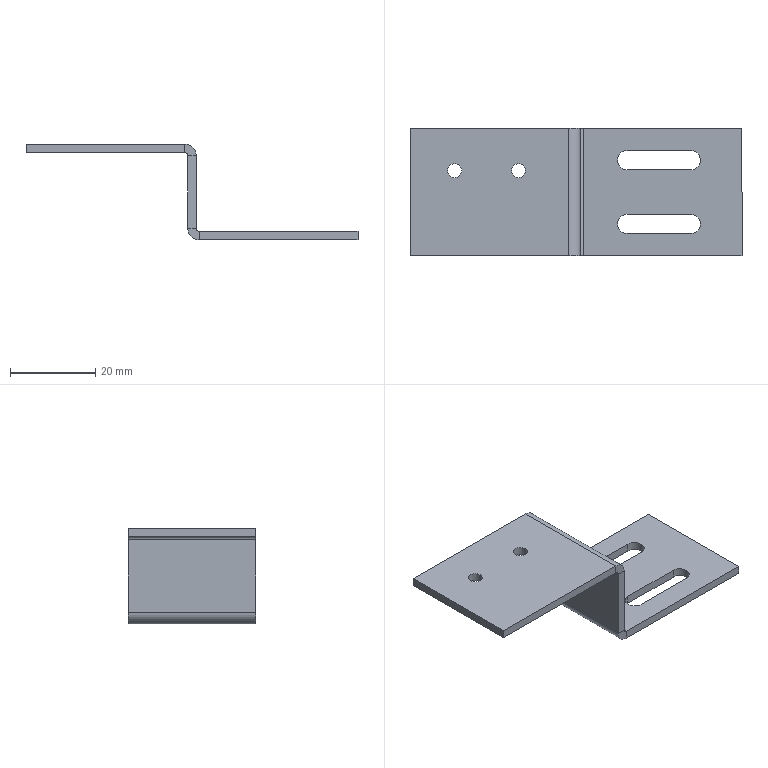Part | SolidWorks | features EdgeFlange 2, FlatPattern 1, HoleWzd 1, ICE 1, SMBaseFlange 1, SheetMetal 1 | 1 solid | 36 faces | box 78 x 30 x 22.5 mm | volume 5453 mm3 | plane 22 | cylinder 14 | commonest cylinder face diameters 4.5 x6 3.3 x4 1.473 x2 5.473 x2
STEP:
#1=CARTESIAN_POINT('',(10.25,-7.5,-2.));
#2=VERTEX_POINT('',#1);
#3=CARTESIAN_POINT('',(8.,-5.25,-2.));
#4=VERTEX_POINT('',#3);
#5=CARTESIAN_POINT('',(8.,-7.5,-2.));
#6=DIRECTION('',(0.,0.,1.));
#7=DIRECTION('',(1.,0.,0.));
#8=AXIS2_PLACEMENT_3D('',#5,#6,#7);
#9=CIRCLE('',#8,2.25);
#10=EDGE_CURVE('',#2,#4,#9,.T.);
#11=ORIENTED_EDGE('',*,*,#10,.F.);
#12=CARTESIAN_POINT('',(10.25,-7.5,0.));
#13=VERTEX_POINT('',#12);
#14=CARTESIAN_POINT('',(10.25,-7.5,-2.));
#15=DIRECTION('',(0.,0.,1.));
#16=VECTOR('',#15,1000.);
#17=LINE('',#14,#16);
#18=EDGE_CURVE('',#2,#13,#17,.T.);
#19=ORIENTED_EDGE('',*,*,#18,.T.);
#20=CARTESIAN_POINT('',(8.,-5.25,0.));
#21=VERTEX_POINT('',#20);
#22=CARTESIAN_POINT('',(8.,-7.5,0.));
#23=DIRECTION('',(0.,0.,1.));
#24=DIRECTION('',(1.,0.,0.));
#25=AXIS2_PLACEMENT_3D('',#22,#23,#24);
#26=CIRCLE('',#25,2.25);
#27=EDGE_CURVE('',#13,#21,#26,.T.);
#28=ORIENTED_EDGE('',*,*,#27,.T.);
#29=CARTESIAN_POINT('',(8.,-5.25,-2.));
#30=DIRECTION('',(0.,0.,1.));
#31=VECTOR('',#30,1000.);
#32=LINE('',#29,#31);
#33=EDGE_CURVE('',#4,#21,#32,.T.);
#34=ORIENTED_EDGE('',*,*,#33,.F.);
#35=EDGE_LOOP('',(#11,#19,#28,#34));
#36=FACE_OUTER_BOUND('',#35,.T.);
#37=CARTESIAN_POINT('',(8.,-7.5,-2.));
#38=DIRECTION('',(0.,0.,1.));
#39=DIRECTION('',(1.,0.,0.));
#40=AXIS2_PLACEMENT_3D('',#37,#38,#39);
#41=CYLINDRICAL_SURFACE('',#40,2.25);
#42=ADVANCED_FACE('',(#36),#41,.F.);
#43=CARTESIAN_POINT('',(10.25,7.5,-2.));
#44=VERTEX_POINT('',#43);
#45=CARTESIAN_POINT('',(8.,9.75,-2.));
#46=VERTEX_POINT('',#45);
#47=CARTESIAN_POINT('',(8.,7.5,-2.));
#48=DIRECTION('',(0.,0.,1.));
#49=DIRECTION('',(1.,0.,0.));
#50=AXIS2_PLACEMENT_3D('',#47,#48,#49);
#51=CIRCLE('',#50,2.25);
#52=EDGE_CURVE('',#44,#46,#51,.T.);
#53=ORIENTED_EDGE('',*,*,#52,.F.);
#54=CARTESIAN_POINT('',(10.25,7.5,0.));
#55=VERTEX_POINT('',#54);
#56=CARTESIAN_POINT('',(10.25,7.5,-2.));
#57=DIRECTION('',(0.,0.,1.));
#58=VECTOR('',#57,1000.);
#59=LINE('',#56,#58);
#60=EDGE_CURVE('',#44,#55,#59,.T.);
#61=ORIENTED_EDGE('',*,*,#60,.T.);
#62=CARTESIAN_POINT('',(8.,9.75,0.));
#63=VERTEX_POINT('',#62);
#64=CARTESIAN_POINT('',(8.,7.5,0.));
#65=DIRECTION('',(0.,0.,1.));
#66=DIRECTION('',(1.,0.,0.));
#67=AXIS2_PLACEMENT_3D('',#64,#65,#66);
#68=CIRCLE('',#67,2.25);
#69=EDGE_CURVE('',#55,#63,#68,.T.);
#70=ORIENTED_EDGE('',*,*,#69,.T.);
#71=CARTESIAN_POINT('',(8.,9.75,-2.));
#72=DIRECTION('',(0.,0.,1.));
#73=VECTOR('',#72,1000.);
#74=LINE('',#71,#73);
#75=EDGE_CURVE('',#46,#63,#74,.T.);
#76=ORIENTED_EDGE('',*,*,#75,.F.);
#77=EDGE_LOOP('',(#53,#61,#70,#76));
#78=FACE_OUTER_BOUND('',#77,.T.);
#79=CARTESIAN_POINT('',(8.,7.5,-2.));
#80=DIRECTION('',(0.,0.,1.));
#81=DIRECTION('',(1.,0.,0.));
#82=AXIS2_PLACEMENT_3D('',#79,#80,#81);
#83=CYLINDRICAL_SURFACE('',#82,2.25);
#84=ADVANCED_FACE('',(#78),#83,.F.);
#85=CARTESIAN_POINT('',(-45.85,5.,18.5));
#86=VERTEX_POINT('',#85);
#87=CARTESIAN_POINT('',(-49.15,5.,18.5));
#88=VERTEX_POINT('',#87);
#89=CARTESIAN_POINT('',(-47.5,5.,18.5));
#90=DIRECTION('',(0.,0.,-1.));
#91=DIRECTION('',(-1.,0.,0.));
#92=AXIS2_PLACEMENT_3D('',#89,#90,#91);
#93=CIRCLE('',#92,1.65);
#94=EDGE_CURVE('',#86,#88,#93,.T.);
#95=ORIENTED_EDGE('',*,*,#94,.T.);
#96=CARTESIAN_POINT('',(-49.15,5.,20.5));
#97=VERTEX_POINT('',#96);
#98=CARTESIAN_POINT('',(-49.15,5.,20.5));
#99=DIRECTION('',(0.,0.,1.));
#100=VECTOR('',#99,1000.);
#101=LINE('',#98,#100);
#102=EDGE_CURVE('',#88,#97,#101,.T.);
#103=ORIENTED_EDGE('',*,*,#102,.T.);
#104=CARTESIAN_POINT('',(-45.85,5.,20.5));
#105=VERTEX_POINT('',#104);
#106=CARTESIAN_POINT('',(-47.5,5.,20.5));
#107=DIRECTION('',(0.,0.,1.));
#108=DIRECTION('',(1.,0.,0.));
#109=AXIS2_PLACEMENT_3D('',#106,#107,#108);
#110=CIRCLE('',#109,1.65);
#111=EDGE_CURVE('',#97,#105,#110,.T.);
#112=ORIENTED_EDGE('',*,*,#111,.T.);
#113=CARTESIAN_POINT('',(-45.85,5.,20.5));
#114=DIRECTION('',(0.,0.,1.));
#115=VECTOR('',#114,1000.);
#116=LINE('',#113,#115);
#117=EDGE_CURVE('',#86,#105,#116,.T.);
#118=ORIENTED_EDGE('',*,*,#117,.F.);
#119=EDGE_LOOP('',(#95,#103,#112,#118));
#120=FACE_OUTER_BOUND('',#119,.T.);
#121=CARTESIAN_POINT('',(-47.5,5.,20.5));
#122=DIRECTION('',(0.,0.,1.));
#123=DIRECTION('',(1.,0.,0.));
#124=AXIS2_PLACEMENT_3D('',#121,#122,#123);
#125=CYLINDRICAL_SURFACE('',#124,1.65);
#126=ADVANCED_FACE('',(#120),#125,.F.);
#127=CARTESIAN_POINT('',(-30.85,5.,18.5));
#128=VERTEX_POINT('',#127);
#129=CARTESIAN_POINT('',(-34.15,5.,18.5));
#130=VERTEX_POINT('',#129);
#131=CARTESIAN_POINT('',(-32.5,5.,18.5));
#132=DIRECTION('',(0.,0.,-1.));
#133=DIRECTION('',(-1.,0.,0.));
#134=AXIS2_PLACEMENT_3D('',#131,#132,#133);
#135=CIRCLE('',#134,1.65);
#136=EDGE_CURVE('',#128,#130,#135,.T.);
#137=ORIENTED_EDGE('',*,*,#136,.T.);
#138=CARTESIAN_POINT('',(-34.15,5.,20.5));
#139=VERTEX_POINT('',#138);
#140=CARTESIAN_POINT('',(-34.15,5.,20.5));
#141=DIRECTION('',(0.,0.,1.));
#142=VECTOR('',#141,1000.);
#143=LINE('',#140,#142);
#144=EDGE_CURVE('',#130,#139,#143,.T.);
#145=ORIENTED_EDGE('',*,*,#144,.T.);
#146=CARTESIAN_POINT('',(-30.85,5.,20.5));
#147=VERTEX_POINT('',#146);
#148=CARTESIAN_POINT('',(-32.5,5.,20.5));
#149=DIRECTION('',(0.,0.,1.));
#150=DIRECTION('',(1.,0.,0.));
#151=AXIS2_PLACEMENT_3D('',#148,#149,#150);
#152=CIRCLE('',#151,1.65);
#153=EDGE_CURVE('',#139,#147,#152,.T.);
#154=ORIENTED_EDGE('',*,*,#153,.T.);
#155=CARTESIAN_POINT('',(-30.85,5.,20.5));
#156=DIRECTION('',(0.,0.,1.));
#157=VECTOR('',#156,1000.);
#158=LINE('',#155,#157);
#159=EDGE_CURVE('',#128,#147,#158,.T.);
#160=ORIENTED_EDGE('',*,*,#159,.F.);
#161=EDGE_LOOP('',(#137,#145,#154,#160));
#162=FACE_OUTER_BOUND('',#161,.T.);
#163=CARTESIAN_POINT('',(-32.5,5.,20.5));
#164=DIRECTION('',(0.,0.,1.));
#165=DIRECTION('',(1.,0.,0.));
#166=AXIS2_PLACEMENT_3D('',#163,#164,#165);
#167=CYLINDRICAL_SURFACE('',#166,1.65);
#168=ADVANCED_FACE('',(#162),#167,.F.);
#169=CARTESIAN_POINT('',(-20.,15.,0.7366));
#170=VERTEX_POINT('',#169);
#171=CARTESIAN_POINT('',(-20.,15.,17.763));
#172=VERTEX_POINT('',#171);
#173=CARTESIAN_POINT('',(-20.,15.,20.5));
#174=DIRECTION('',(0.,0.,1.));
#175=VECTOR('',#174,1000.);
#176=LINE('',#173,#175);
#177=EDGE_CURVE('',#170,#172,#176,.T.);
#178=ORIENTED_EDGE('',*,*,#177,.T.);
#179=CARTESIAN_POINT('',(-18.,15.,17.763));
#180=VERTEX_POINT('',#179);
#181=CARTESIAN_POINT('',(-20.,15.,17.763));
#182=DIRECTION('',(1.,0.,0.));
#183=VECTOR('',#182,1000.);
#184=LINE('',#181,#183);
#185=EDGE_CURVE('',#172,#180,#184,.T.);
#186=ORIENTED_EDGE('',*,*,#185,.T.);
#187=CARTESIAN_POINT('',(-18.,15.,0.7366));
#188=VERTEX_POINT('',#187);
#189=CARTESIAN_POINT('',(-18.,15.,0.));
#190=DIRECTION('',(0.,0.,1.));
#191=VECTOR('',#190,1000.);
#192=LINE('',#189,#191);
#193=EDGE_CURVE('',#188,#180,#192,.T.);
#194=ORIENTED_EDGE('',*,*,#193,.F.);
#195=CARTESIAN_POINT('',(-20.,15.,0.7366));
#196=DIRECTION('',(-1.,0.,0.));
#197=VECTOR('',#196,1000.);
#198=LINE('',#195,#197);
#199=EDGE_CURVE('',#188,#170,#198,.T.);
#200=ORIENTED_EDGE('',*,*,#199,.T.);
#201=EDGE_LOOP('',(#178,#186,#194,#200));
#202=FACE_OUTER_BOUND('',#201,.T.);
#203=CARTESIAN_POINT('',(-20.,15.,20.5));
#204=DIRECTION('',(0.,1.,0.));
#205=DIRECTION('',(0.,0.,1.));
#206=AXIS2_PLACEMENT_3D('',#203,#204,#205);
#207=PLANE('',#206);
#208=ADVANCED_FACE('',(#202),#207,.T.);
#209=CARTESIAN_POINT('',(-20.,-15.,17.763));
#210=VERTEX_POINT('',#209);
#211=CARTESIAN_POINT('',(-20.,-15.,0.7366));
#212=VERTEX_POINT('',#211);
#213=CARTESIAN_POINT('',(-20.,-15.,0.));
#214=DIRECTION('',(0.,0.,-1.));
#215=VECTOR('',#214,1000.);
#216=LINE('',#213,#215);
#217=EDGE_CURVE('',#210,#212,#216,.T.);
#218=ORIENTED_EDGE('',*,*,#217,.F.);
#219=CARTESIAN_POINT('',(-20.,15.,17.763));
#220=DIRECTION('',(0.,-1.,0.));
#221=VECTOR('',#220,1000.);
#222=LINE('',#219,#221);
#223=EDGE_CURVE('',#172,#210,#222,.T.);
#224=ORIENTED_EDGE('',*,*,#223,.F.);
#225=ORIENTED_EDGE('',*,*,#177,.F.);
#226=CARTESIAN_POINT('',(-20.,0.,0.7366));
#227=DIRECTION('',(0.,-1.,0.));
#228=VECTOR('',#227,1000.);
#229=LINE('',#226,#228);
#230=EDGE_CURVE('',#170,#212,#229,.T.);
#231=ORIENTED_EDGE('',*,*,#230,.T.);
#232=EDGE_LOOP('',(#218,#224,#225,#231));
#233=FACE_OUTER_BOUND('',#232,.T.);
#234=CARTESIAN_POINT('',(-20.,0.,0.));
#235=DIRECTION('',(-1.,0.,0.));
#236=DIRECTION('',(0.,0.,1.));
#237=AXIS2_PLACEMENT_3D('',#234,#235,#236);
#238=PLANE('',#237);
#239=ADVANCED_FACE('',(#233),#238,.T.);
#240=CARTESIAN_POINT('',(-18.,-15.,17.763));
#241=VERTEX_POINT('',#240);
#242=CARTESIAN_POINT('',(-18.,15.,17.763));
#243=DIRECTION('',(0.,-1.,0.));
#244=VECTOR('',#243,1000.);
#245=LINE('',#242,#244);
#246=EDGE_CURVE('',#180,#241,#245,.T.);
#247=ORIENTED_EDGE('',*,*,#246,.T.);
#248=CARTESIAN_POINT('',(-18.,-15.,0.7366));
#249=VERTEX_POINT('',#248);
#250=CARTESIAN_POINT('',(-18.,-15.,0.));
#251=DIRECTION('',(0.,0.,-1.));
#252=VECTOR('',#251,1000.);
#253=LINE('',#250,#252);
#254=EDGE_CURVE('',#241,#249,#253,.T.);
#255=ORIENTED_EDGE('',*,*,#254,.T.);
#256=CARTESIAN_POINT('',(-18.,15.,0.7366));
#257=DIRECTION('',(0.,-1.,0.));
#258=VECTOR('',#257,1000.);
#259=LINE('',#256,#258);
#260=EDGE_CURVE('',#188,#249,#259,.T.);
#261=ORIENTED_EDGE('',*,*,#260,.F.);
#262=ORIENTED_EDGE('',*,*,#193,.T.);
#263=EDGE_LOOP('',(#247,#255,#261,#262));
#264=FACE_OUTER_BOUND('',#263,.T.);
#265=CARTESIAN_POINT('',(-18.,0.,0.));
#266=DIRECTION('',(-1.,0.,0.));
#267=DIRECTION('',(0.,0.,1.));
#268=AXIS2_PLACEMENT_3D('',#265,#266,#267);
#269=PLANE('',#268);
#270=ADVANCED_FACE('',(#264),#269,.F.);
#271=CARTESIAN_POINT('',(-17.263,-15.,0.));
#272=VERTEX_POINT('',#271);
#273=CARTESIAN_POINT('',(20.,-15.,0.));
#274=VERTEX_POINT('',#273);
#275=CARTESIAN_POINT('',(-20.,-15.,0.));
#276=DIRECTION('',(1.,0.,0.));
#277=VECTOR('',#276,1000.);
#278=LINE('',#275,#277);
#279=EDGE_CURVE('',#272,#274,#278,.T.);
#280=ORIENTED_EDGE('',*,*,#279,.F.);
#281=CARTESIAN_POINT('',(-17.263,-15.,-2.));
#282=VERTEX_POINT('',#281);
#283=CARTESIAN_POINT('',(-17.263,-15.,0.));
#284=DIRECTION('',(0.,0.,-1.));
#285=VECTOR('',#284,1000.);
#286=LINE('',#283,#285);
#287=EDGE_CURVE('',#272,#282,#286,.T.);
#288=ORIENTED_EDGE('',*,*,#287,.T.);
#289=CARTESIAN_POINT('',(20.,-15.,-2.));
#290=VERTEX_POINT('',#289);
#291=CARTESIAN_POINT('',(-20.,-15.,-2.));
#292=DIRECTION('',(1.,0.,0.));
#293=VECTOR('',#292,1000.);
#294=LINE('',#291,#293);
#295=EDGE_CURVE('',#282,#290,#294,.T.);
#296=ORIENTED_EDGE('',*,*,#295,.T.);
#297=CARTESIAN_POINT('',(20.,-15.,-2.));
#298=DIRECTION('',(0.,0.,1.));
#299=VECTOR('',#298,1000.);
#300=LINE('',#297,#299);
#301=EDGE_CURVE('',#290,#274,#300,.T.);
#302=ORIENTED_EDGE('',*,*,#301,.T.);
#303=EDGE_LOOP('',(#280,#288,#296,#302));
#304=FACE_OUTER_BOUND('',#303,.T.);
#305=CARTESIAN_POINT('',(-20.,-15.,-2.));
#306=DIRECTION('',(0.,-1.,0.));
#307=DIRECTION('',(0.,0.,-1.));
#308=AXIS2_PLACEMENT_3D('',#305,#306,#307);
#309=PLANE('',#308);
#310=ADVANCED_FACE('',(#304),#309,.T.);
#311=CARTESIAN_POINT('',(-7.,-5.25,-2.));
#312=VERTEX_POINT('',#311);
#313=CARTESIAN_POINT('',(-7.,-5.25,-2.));
#314=DIRECTION('',(-1.,0.,0.));
#315=VECTOR('',#314,1000.);
#316=LINE('',#313,#315);
#317=EDGE_CURVE('',#4,#312,#316,.T.);
#318=ORIENTED_EDGE('',*,*,#317,.T.);
#319=CARTESIAN_POINT('',(-7.,-9.75,-2.));
#320=VERTEX_POINT('',#319);
#321=CARTESIAN_POINT('',(-7.,-7.5,-2.));
#322=DIRECTION('',(0.,0.,1.));
#323=DIRECTION('',(1.,0.,0.));
#324=AXIS2_PLACEMENT_3D('',#321,#322,#323);
#325=CIRCLE('',#324,2.25);
#326=EDGE_CURVE('',#312,#320,#325,.T.);
#327=ORIENTED_EDGE('',*,*,#326,.T.);
#328=CARTESIAN_POINT('',(8.,-9.75,-2.));
#329=VERTEX_POINT('',#328);
#330=CARTESIAN_POINT('',(-7.,-9.75,-2.));
#331=DIRECTION('',(1.,0.,0.));
#332=VECTOR('',#331,1000.);
#333=LINE('',#330,#332);
#334=EDGE_CURVE('',#320,#329,#333,.T.);
#335=ORIENTED_EDGE('',*,*,#334,.T.);
#336=CARTESIAN_POINT('',(8.,-7.5,-2.));
#337=DIRECTION('',(0.,0.,1.));
#338=DIRECTION('',(1.,0.,0.));
#339=AXIS2_PLACEMENT_3D('',#336,#337,#338);
#340=CIRCLE('',#339,2.25);
#341=EDGE_CURVE('',#329,#2,#340,.T.);
#342=ORIENTED_EDGE('',*,*,#341,.T.);
#343=ORIENTED_EDGE('',*,*,#10,.T.);
#344=EDGE_LOOP('',(#318,#327,#335,#342,#343));
#345=FACE_BOUND('',#344,.T.);
#346=CARTESIAN_POINT('',(-7.,9.75,-2.));
#347=VERTEX_POINT('',#346);
#348=CARTESIAN_POINT('',(-7.,9.75,-2.));
#349=DIRECTION('',(-1.,0.,0.));
#350=VECTOR('',#349,1000.);
#351=LINE('',#348,#350);
#352=EDGE_CURVE('',#46,#347,#351,.T.);
#353=ORIENTED_EDGE('',*,*,#352,.T.);
#354=CARTESIAN_POINT('',(-7.,5.25,-2.));
#355=VERTEX_POINT('',#354);
#356=CARTESIAN_POINT('',(-7.,7.5,-2.));
#357=DIRECTION('',(0.,0.,1.));
#358=DIRECTION('',(1.,0.,0.));
#359=AXIS2_PLACEMENT_3D('',#356,#357,#358);
#360=CIRCLE('',#359,2.25);
#361=EDGE_CURVE('',#347,#355,#360,.T.);
#362=ORIENTED_EDGE('',*,*,#361,.T.);
#363=CARTESIAN_POINT('',(8.,5.25,-2.));
#364=VERTEX_POINT('',#363);
#365=CARTESIAN_POINT('',(-7.,5.25,-2.));
#366=DIRECTION('',(1.,0.,0.));
#367=VECTOR('',#366,1000.);
#368=LINE('',#365,#367);
#369=EDGE_CURVE('',#355,#364,#368,.T.);
#370=ORIENTED_EDGE('',*,*,#369,.T.);
#371=CARTESIAN_POINT('',(8.,7.5,-2.));
#372=DIRECTION('',(0.,0.,1.));
#373=DIRECTION('',(1.,0.,0.));
#374=AXIS2_PLACEMENT_3D('',#371,#372,#373);
#375=CIRCLE('',#374,2.25);
#376=EDGE_CURVE('',#364,#44,#375,.T.);
#377=ORIENTED_EDGE('',*,*,#376,.T.);
#378=ORIENTED_EDGE('',*,*,#52,.T.);
#379=EDGE_LOOP('',(#353,#362,#370,#377,#378));
#380=FACE_BOUND('',#379,.T.);
#381=CARTESIAN_POINT('',(-17.263,15.,-2.));
#382=VERTEX_POINT('',#381);
#383=CARTESIAN_POINT('',(-17.263,-15.,-2.));
#384=DIRECTION('',(0.,1.,0.));
#385=VECTOR('',#384,1000.);
#386=LINE('',#383,#385);
#387=EDGE_CURVE('',#282,#382,#386,.T.);
#388=ORIENTED_EDGE('',*,*,#387,.T.);
#389=CARTESIAN_POINT('',(20.,15.,-2.));
#390=VERTEX_POINT('',#389);
#391=CARTESIAN_POINT('',(-20.,15.,-2.));
#392=DIRECTION('',(-1.,0.,0.));
#393=VECTOR('',#392,1000.);
#394=LINE('',#391,#393);
#395=EDGE_CURVE('',#390,#382,#394,.T.);
#396=ORIENTED_EDGE('',*,*,#395,.F.);
#397=CARTESIAN_POINT('',(20.,15.,-2.));
#398=DIRECTION('',(0.,1.,0.));
#399=VECTOR('',#398,1000.);
#400=LINE('',#397,#399);
#401=EDGE_CURVE('',#290,#390,#400,.T.);
#402=ORIENTED_EDGE('',*,*,#401,.F.);
#403=ORIENTED_EDGE('',*,*,#295,.F.);
#404=EDGE_LOOP('',(#388,#396,#402,#403));
#405=FACE_OUTER_BOUND('',#404,.T.);
#406=CARTESIAN_POINT('',(0.,0.,-2.));
#407=DIRECTION('',(0.,0.,1.));
#408=DIRECTION('',(1.,0.,0.));
#409=AXIS2_PLACEMENT_3D('',#406,#407,#408);
#410=PLANE('',#409);
#411=ADVANCED_FACE('',(#345,#380,#405),#410,.F.);
#412=CARTESIAN_POINT('',(-7.,-5.25,0.));
#413=VERTEX_POINT('',#412);
#414=CARTESIAN_POINT('',(-7.,-9.75,0.));
#415=VERTEX_POINT('',#414);
#416=CARTESIAN_POINT('',(-7.,-7.5,0.));
#417=DIRECTION('',(0.,0.,1.));
#418=DIRECTION('',(1.,0.,0.));
#419=AXIS2_PLACEMENT_3D('',#416,#417,#418);
#420=CIRCLE('',#419,2.25);
#421=EDGE_CURVE('',#413,#415,#420,.T.);
#422=ORIENTED_EDGE('',*,*,#421,.F.);
#423=CARTESIAN_POINT('',(-7.,-5.25,0.));
#424=DIRECTION('',(-1.,0.,0.));
#425=VECTOR('',#424,1000.);
#426=LINE('',#423,#425);
#427=EDGE_CURVE('',#21,#413,#426,.T.);
#428=ORIENTED_EDGE('',*,*,#427,.F.);
#429=ORIENTED_EDGE('',*,*,#27,.F.);
#430=CARTESIAN_POINT('',(8.,-9.75,0.));
#431=VERTEX_POINT('',#430);
#432=CARTESIAN_POINT('',(8.,-7.5,0.));
#433=DIRECTION('',(0.,0.,1.));
#434=DIRECTION('',(1.,0.,0.));
#435=AXIS2_PLACEMENT_3D('',#432,#433,#434);
#436=CIRCLE('',#435,2.25);
#437=EDGE_CURVE('',#431,#13,#436,.T.);
#438=ORIENTED_EDGE('',*,*,#437,.F.);
#439=CARTESIAN_POINT('',(-7.,-9.75,0.));
#440=DIRECTION('',(1.,0.,0.));
#441=VECTOR('',#440,1000.);
#442=LINE('',#439,#441);
#443=EDGE_CURVE('',#415,#431,#442,.T.);
#444=ORIENTED_EDGE('',*,*,#443,.F.);
#445=EDGE_LOOP('',(#422,#428,#429,#438,#444));
#446=FACE_BOUND('',#445,.T.);
#447=CARTESIAN_POINT('',(-7.,9.75,0.));
#448=VERTEX_POINT('',#447);
#449=CARTESIAN_POINT('',(-7.,5.25,0.));
#450=VERTEX_POINT('',#449);
#451=CARTESIAN_POINT('',(-7.,7.5,0.));
#452=DIRECTION('',(0.,0.,1.));
#453=DIRECTION('',(1.,0.,0.));
#454=AXIS2_PLACEMENT_3D('',#451,#452,#453);
#455=CIRCLE('',#454,2.25);
#456=EDGE_CURVE('',#448,#450,#455,.T.);
#457=ORIENTED_EDGE('',*,*,#456,.F.);
#458=CARTESIAN_POINT('',(-7.,9.75,0.));
#459=DIRECTION('',(-1.,0.,0.));
#460=VECTOR('',#459,1000.);
#461=LINE('',#458,#460);
#462=EDGE_CURVE('',#63,#448,#461,.T.);
#463=ORIENTED_EDGE('',*,*,#462,.F.);
#464=ORIENTED_EDGE('',*,*,#69,.F.);
#465=CARTESIAN_POINT('',(8.,5.25,0.));
#466=VERTEX_POINT('',#465);
#467=CARTESIAN_POINT('',(8.,7.5,0.));
#468=DIRECTION('',(0.,0.,1.));
#469=DIRECTION('',(1.,0.,0.));
#470=AXIS2_PLACEMENT_3D('',#467,#468,#469);
#471=CIRCLE('',#470,2.25);
#472=EDGE_CURVE('',#466,#55,#471,.T.);
#473=ORIENTED_EDGE('',*,*,#472,.F.);
#474=CARTESIAN_POINT('',(-7.,5.25,0.));
#475=DIRECTION('',(1.,0.,0.));
#476=VECTOR('',#475,1000.);
#477=LINE('',#474,#476);
#478=EDGE_CURVE('',#450,#466,#477,.T.);
#479=ORIENTED_EDGE('',*,*,#478,.F.);
#480=EDGE_LOOP('',(#457,#463,#464,#473,#479));
#481=FACE_BOUND('',#480,.T.);
#482=CARTESIAN_POINT('',(20.,15.,0.));
#483=VERTEX_POINT('',#482);
#484=CARTESIAN_POINT('',(-17.263,15.,0.));
#485=VERTEX_POINT('',#484);
#486=CARTESIAN_POINT('',(-20.,15.,0.));
#487=DIRECTION('',(-1.,0.,0.));
#488=VECTOR('',#487,1000.);
#489=LINE('',#486,#488);
#490=EDGE_CURVE('',#483,#485,#489,.T.);
#491=ORIENTED_EDGE('',*,*,#490,.T.);
#492=CARTESIAN_POINT('',(-17.263,-15.,0.));
#493=DIRECTION('',(0.,1.,0.));
#494=VECTOR('',#493,1000.);
#495=LINE('',#492,#494);
#496=EDGE_CURVE('',#272,#485,#495,.T.);
#497=ORIENTED_EDGE('',*,*,#496,.F.);
#498=ORIENTED_EDGE('',*,*,#279,.T.);
#499=CARTESIAN_POINT('',(20.,15.,0.));
#500=DIRECTION('',(0.,1.,0.));
#501=VECTOR('',#500,1000.);
#502=LINE('',#499,#501);
#503=EDGE_CURVE('',#274,#483,#502,.T.);
#504=ORIENTED_EDGE('',*,*,#503,.T.);
#505=EDGE_LOOP('',(#491,#497,#498,#504));
#506=FACE_OUTER_BOUND('',#505,.T.);
#507=CARTESIAN_POINT('',(0.,0.,0.));
#508=DIRECTION('',(0.,0.,1.));
#509=DIRECTION('',(1.,0.,0.));
#510=AXIS2_PLACEMENT_3D('',#507,#508,#509);
#511=PLANE('',#510);
#512=ADVANCED_FACE('',(#446,#481,#506),#511,.T.);
#513=ORIENTED_EDGE('',*,*,#503,.F.);
#514=ORIENTED_EDGE('',*,*,#301,.F.);
#515=ORIENTED_EDGE('',*,*,#401,.T.);
#516=CARTESIAN_POINT('',(20.,15.,-2.));
#517=DIRECTION('',(0.,0.,1.));
#518=VECTOR('',#517,1000.);
#519=LINE('',#516,#518);
#520=EDGE_CURVE('',#390,#483,#519,.T.);
#521=ORIENTED_EDGE('',*,*,#520,.T.);
#522=EDGE_LOOP('',(#513,#514,#515,#521));
#523=FACE_OUTER_BOUND('',#522,.T.);
#524=CARTESIAN_POINT('',(20.,15.,-2.));
#525=DIRECTION('',(1.,0.,0.));
#526=DIRECTION('',(0.,1.,0.));
#527=AXIS2_PLACEMENT_3D('',#524,#525,#526);
#528=PLANE('',#527);
#529=ADVANCED_FACE('',(#523),#528,.T.);
#530=CARTESIAN_POINT('',(-17.263,15.,0.));
#531=DIRECTION('',(0.,0.,-1.));
#532=VECTOR('',#531,1000.);
#533=LINE('',#530,#532);
#534=EDGE_CURVE('',#485,#382,#533,.T.);
#535=ORIENTED_EDGE('',*,*,#534,.F.);
#536=ORIENTED_EDGE('',*,*,#490,.F.);
#537=ORIENTED_EDGE('',*,*,#520,.F.);
#538=ORIENTED_EDGE('',*,*,#395,.T.);
#539=EDGE_LOOP('',(#535,#536,#537,#538));
#540=FACE_OUTER_BOUND('',#539,.T.);
#541=CARTESIAN_POINT('',(-20.,15.,-2.));
#542=DIRECTION('',(0.,1.,0.));
#543=DIRECTION('',(0.,0.,1.));
#544=AXIS2_PLACEMENT_3D('',#541,#542,#543);
#545=PLANE('',#544);
#546=ADVANCED_FACE('',(#540),#545,.T.);
#547=ORIENTED_EDGE('',*,*,#199,.F.);
#548=CARTESIAN_POINT('',(-17.263,15.,0.7366));
#549=DIRECTION('',(0.,1.,0.));
#550=DIRECTION('',(0.,0.,-1.));
#551=AXIS2_PLACEMENT_3D('',#548,#549,#550);
#552=CIRCLE('',#551,0.7366);
#553=EDGE_CURVE('',#485,#188,#552,.T.);
#554=ORIENTED_EDGE('',*,*,#553,.F.);
#555=ORIENTED_EDGE('',*,*,#534,.T.);
#556=CARTESIAN_POINT('',(-17.263,15.,0.7366));
#557=DIRECTION('',(0.,1.,0.));
#558=DIRECTION('',(0.,0.,-1.));
#559=AXIS2_PLACEMENT_3D('',#556,#557,#558);
#560=CIRCLE('',#559,2.737);
#561=EDGE_CURVE('',#382,#170,#560,.T.);
#562=ORIENTED_EDGE('',*,*,#561,.T.);
#563=EDGE_LOOP('',(#547,#554,#555,#562));
#564=FACE_OUTER_BOUND('',#563,.T.);
#565=CARTESIAN_POINT('',(-17.263,15.,0.7366));
#566=DIRECTION('',(0.,1.,0.));
#567=DIRECTION('',(0.,0.,1.));
#568=AXIS2_PLACEMENT_3D('',#565,#566,#567);
#569=PLANE('',#568);
#570=ADVANCED_FACE('',(#564),#569,.T.);
#571=CARTESIAN_POINT('',(-17.263,-15.,0.7366));
#572=DIRECTION('',(0.,-1.,0.));
#573=DIRECTION('',(0.,0.,-1.));
#574=AXIS2_PLACEMENT_3D('',#571,#572,#573);
#575=CIRCLE('',#574,0.7366);
#576=EDGE_CURVE('',#249,#272,#575,.T.);
#577=ORIENTED_EDGE('',*,*,#576,.F.);
#578=CARTESIAN_POINT('',(-18.,-15.,0.7366));
#579=DIRECTION('',(-1.,0.,0.));
#580=VECTOR('',#579,1000.);
#581=LINE('',#578,#580);
#582=EDGE_CURVE('',#249,#212,#581,.T.);
#583=ORIENTED_EDGE('',*,*,#582,.T.);
#584=CARTESIAN_POINT('',(-17.263,-15.,0.7366));
#585=DIRECTION('',(0.,-1.,0.));
#586=DIRECTION('',(0.,0.,-1.));
#587=AXIS2_PLACEMENT_3D('',#584,#585,#586);
#588=CIRCLE('',#587,2.737);
#589=EDGE_CURVE('',#212,#282,#588,.T.);
#590=ORIENTED_EDGE('',*,*,#589,.T.);
#591=ORIENTED_EDGE('',*,*,#287,.F.);
#592=EDGE_LOOP('',(#577,#583,#590,#591));
#593=FACE_OUTER_BOUND('',#592,.T.);
#594=CARTESIAN_POINT('',(-17.263,-15.,0.7366));
#595=DIRECTION('',(0.,1.,0.));
#596=DIRECTION('',(0.,0.,1.));
#597=AXIS2_PLACEMENT_3D('',#594,#595,#596);
#598=PLANE('',#597);
#599=ADVANCED_FACE('',(#593),#598,.F.);
#600=ORIENTED_EDGE('',*,*,#387,.F.);
#601=ORIENTED_EDGE('',*,*,#589,.F.);
#602=ORIENTED_EDGE('',*,*,#230,.F.);
#603=ORIENTED_EDGE('',*,*,#561,.F.);
#604=EDGE_LOOP('',(#600,#601,#602,#603));
#605=FACE_OUTER_BOUND('',#604,.T.);
#606=CARTESIAN_POINT('',(-17.263,-15.,0.7366));
#607=DIRECTION('',(0.,-1.,0.));
#608=DIRECTION('',(-1.,0.,0.));
#609=AXIS2_PLACEMENT_3D('',#606,#607,#608);
#610=CYLINDRICAL_SURFACE('',#609,2.737);
#611=ADVANCED_FACE('',(#605),#610,.T.);
#612=ORIENTED_EDGE('',*,*,#496,.T.);
#613=ORIENTED_EDGE('',*,*,#553,.T.);
#614=ORIENTED_EDGE('',*,*,#260,.T.);
#615=ORIENTED_EDGE('',*,*,#576,.T.);
#616=EDGE_LOOP('',(#612,#613,#614,#615));
#617=FACE_OUTER_BOUND('',#616,.T.);
#618=CARTESIAN_POINT('',(-17.263,-15.,0.7366));
#619=DIRECTION('',(0.,-1.,0.));
#620=DIRECTION('',(-1.,0.,0.));
#621=AXIS2_PLACEMENT_3D('',#618,#619,#620);
#622=CYLINDRICAL_SURFACE('',#621,0.7366);
#623=ADVANCED_FACE('',(#617),#622,.F.);
#624=CARTESIAN_POINT('',(-20.,-15.,17.763));
#625=DIRECTION('',(1.,0.,0.));
#626=VECTOR('',#625,1000.);
#627=LINE('',#624,#626);
#628=EDGE_CURVE('',#210,#241,#627,.T.);
#629=ORIENTED_EDGE('',*,*,#628,.F.);
#630=ORIENTED_EDGE('',*,*,#217,.T.);
#631=ORIENTED_EDGE('',*,*,#582,.F.);
#632=ORIENTED_EDGE('',*,*,#254,.F.);
#633=EDGE_LOOP('',(#629,#630,#631,#632));
#634=FACE_OUTER_BOUND('',#633,.T.);
#635=CARTESIAN_POINT('',(-20.,-15.,0.));
#636=DIRECTION('',(0.,-1.,0.));
#637=DIRECTION('',(0.,0.,-1.));
#638=AXIS2_PLACEMENT_3D('',#635,#636,#637);
#639=PLANE('',#638);
#640=ADVANCED_FACE('',(#634),#639,.T.);
#641=CARTESIAN_POINT('',(-20.737,-15.,18.5));
#642=VERTEX_POINT('',#641);
#643=CARTESIAN_POINT('',(-20.737,-15.,20.5));
#644=VERTEX_POINT('',#643);
#645=CARTESIAN_POINT('',(-20.737,-15.,20.5));
#646=DIRECTION('',(0.,0.,1.));
#647=VECTOR('',#646,1000.);
#648=LINE('',#645,#647);
#649=EDGE_CURVE('',#642,#644,#648,.T.);
#650=ORIENTED_EDGE('',*,*,#649,.F.);
#651=CARTESIAN_POINT('',(-20.737,-15.,17.763));
#652=DIRECTION('',(0.,-1.,0.));
#653=DIRECTION('',(0.,0.,1.));
#654=AXIS2_PLACEMENT_3D('',#651,#652,#653);
#655=CIRCLE('',#654,0.7366);
#656=EDGE_CURVE('',#210,#642,#655,.T.);
#657=ORIENTED_EDGE('',*,*,#656,.F.);
#658=ORIENTED_EDGE('',*,*,#628,.T.);
#659=CARTESIAN_POINT('',(-20.737,-15.,17.763));
#660=DIRECTION('',(0.,-1.,0.));
#661=DIRECTION('',(0.,0.,1.));
#662=AXIS2_PLACEMENT_3D('',#659,#660,#661);
#663=CIRCLE('',#662,2.737);
#664=EDGE_CURVE('',#241,#644,#663,.T.);
#665=ORIENTED_EDGE('',*,*,#664,.T.);
#666=EDGE_LOOP('',(#650,#657,#658,#665));
#667=FACE_OUTER_BOUND('',#666,.T.);
#668=CARTESIAN_POINT('',(-20.737,-15.,17.763));
#669=DIRECTION('',(0.,-1.,0.));
#670=DIRECTION('',(0.,0.,-1.));
#671=AXIS2_PLACEMENT_3D('',#668,#669,#670);
#672=PLANE('',#671);
#673=ADVANCED_FACE('',(#667),#672,.T.);
#674=CARTESIAN_POINT('',(-20.737,15.,18.5));
#675=VERTEX_POINT('',#674);
#676=CARTESIAN_POINT('',(-20.737,15.,17.763));
#677=DIRECTION('',(0.,1.,0.));
#678=DIRECTION('',(0.,0.,1.));
#679=AXIS2_PLACEMENT_3D('',#676,#677,#678);
#680=CIRCLE('',#679,0.7366);
#681=EDGE_CURVE('',#675,#172,#680,.T.);
#682=ORIENTED_EDGE('',*,*,#681,.F.);
#683=CARTESIAN_POINT('',(-20.737,15.,20.5));
#684=VERTEX_POINT('',#683);
#685=CARTESIAN_POINT('',(-20.737,15.,18.5));
#686=DIRECTION('',(0.,0.,1.));
#687=VECTOR('',#686,1000.);
#688=LINE('',#685,#687);
#689=EDGE_CURVE('',#675,#684,#688,.T.);
#690=ORIENTED_EDGE('',*,*,#689,.T.);
#691=CARTESIAN_POINT('',(-20.737,15.,17.763));
#692=DIRECTION('',(0.,1.,0.));
#693=DIRECTION('',(0.,0.,1.));
#694=AXIS2_PLACEMENT_3D('',#691,#692,#693);
#695=CIRCLE('',#694,2.737);
#696=EDGE_CURVE('',#684,#180,#695,.T.);
#697=ORIENTED_EDGE('',*,*,#696,.T.);
#698=ORIENTED_EDGE('',*,*,#185,.F.);
#699=EDGE_LOOP('',(#682,#690,#697,#698));
#700=FACE_OUTER_BOUND('',#699,.T.);
#701=CARTESIAN_POINT('',(-20.737,15.,17.763));
#702=DIRECTION('',(0.,-1.,0.));
#703=DIRECTION('',(0.,0.,-1.));
#704=AXIS2_PLACEMENT_3D('',#701,#702,#703);
#705=PLANE('',#704);
#706=ADVANCED_FACE('',(#700),#705,.F.);
#707=ORIENTED_EDGE('',*,*,#246,.F.);
#708=ORIENTED_EDGE('',*,*,#696,.F.);
#709=CARTESIAN_POINT('',(-20.737,-15.,20.5));
#710=DIRECTION('',(0.,-1.,0.));
#711=VECTOR('',#710,1000.);
#712=LINE('',#709,#711);
#713=EDGE_CURVE('',#684,#644,#712,.T.);
#714=ORIENTED_EDGE('',*,*,#713,.T.);
#715=ORIENTED_EDGE('',*,*,#664,.F.);
#716=EDGE_LOOP('',(#707,#708,#714,#715));
#717=FACE_OUTER_BOUND('',#716,.T.);
#718=CARTESIAN_POINT('',(-20.737,15.,17.763));
#719=DIRECTION('',(0.,1.,0.));
#720=DIRECTION('',(0.,0.,1.));
#721=AXIS2_PLACEMENT_3D('',#718,#719,#720);
#722=CYLINDRICAL_SURFACE('',#721,2.737);
#723=ADVANCED_FACE('',(#717),#722,.T.);
#724=ORIENTED_EDGE('',*,*,#223,.T.);
#725=ORIENTED_EDGE('',*,*,#656,.T.);
#726=CARTESIAN_POINT('',(-20.737,-15.,18.5));
#727=DIRECTION('',(0.,1.,0.));
#728=VECTOR('',#727,1000.);
#729=LINE('',#726,#728);
#730=EDGE_CURVE('',#642,#675,#729,.T.);
#731=ORIENTED_EDGE('',*,*,#730,.T.);
#732=ORIENTED_EDGE('',*,*,#681,.T.);
#733=EDGE_LOOP('',(#724,#725,#731,#732));
#734=FACE_OUTER_BOUND('',#733,.T.);
#735=CARTESIAN_POINT('',(-20.737,15.,17.763));
#736=DIRECTION('',(0.,1.,0.));
#737=DIRECTION('',(0.,0.,1.));
#738=AXIS2_PLACEMENT_3D('',#735,#736,#737);
#739=CYLINDRICAL_SURFACE('',#738,0.7366);
#740=ADVANCED_FACE('',(#734),#739,.F.);
#741=ORIENTED_EDGE('',*,*,#689,.F.);
#742=CARTESIAN_POINT('',(-58.,15.,18.5));
#743=VERTEX_POINT('',#742);
#744=CARTESIAN_POINT('',(-58.,15.,18.5));
#745=DIRECTION('',(-1.,0.,0.));
#746=VECTOR('',#745,1000.);
#747=LINE('',#744,#746);
#748=EDGE_CURVE('',#675,#743,#747,.T.);
#749=ORIENTED_EDGE('',*,*,#748,.T.);
#750=CARTESIAN_POINT('',(-58.,15.,20.5));
#751=VERTEX_POINT('',#750);
#752=CARTESIAN_POINT('',(-58.,15.,20.5));
#753=DIRECTION('',(0.,0.,-1.));
#754=VECTOR('',#753,1000.);
#755=LINE('',#752,#754);
#756=EDGE_CURVE('',#751,#743,#755,.T.);
#757=ORIENTED_EDGE('',*,*,#756,.F.);
#758=CARTESIAN_POINT('',(0.,15.,20.5));
#759=DIRECTION('',(-1.,0.,0.));
#760=VECTOR('',#759,1000.);
#761=LINE('',#758,#760);
#762=EDGE_CURVE('',#684,#751,#761,.T.);
#763=ORIENTED_EDGE('',*,*,#762,.F.);
#764=EDGE_LOOP('',(#741,#749,#757,#763));
#765=FACE_OUTER_BOUND('',#764,.T.);
#766=CARTESIAN_POINT('',(-58.,15.,20.5));
#767=DIRECTION('',(0.,-1.,0.));
#768=DIRECTION('',(0.,0.,-1.));
#769=AXIS2_PLACEMENT_3D('',#766,#767,#768);
#770=PLANE('',#769);
#771=ADVANCED_FACE('',(#765),#770,.F.);
#772=ORIENTED_EDGE('',*,*,#649,.T.);
#773=CARTESIAN_POINT('',(-58.,-15.,20.5));
#774=VERTEX_POINT('',#773);
#775=CARTESIAN_POINT('',(0.,-15.,20.5));
#776=DIRECTION('',(1.,0.,0.));
#777=VECTOR('',#776,1000.);
#778=LINE('',#775,#777);
#779=EDGE_CURVE('',#774,#644,#778,.T.);
#780=ORIENTED_EDGE('',*,*,#779,.F.);
#781=CARTESIAN_POINT('',(-58.,-15.,18.5));
#782=VERTEX_POINT('',#781);
#783=CARTESIAN_POINT('',(-58.,-15.,20.5));
#784=DIRECTION('',(0.,0.,-1.));
#785=VECTOR('',#784,1000.);
#786=LINE('',#783,#785);
#787=EDGE_CURVE('',#774,#782,#786,.T.);
#788=ORIENTED_EDGE('',*,*,#787,.T.);
#789=CARTESIAN_POINT('',(-20.,-15.,18.5));
#790=DIRECTION('',(1.,0.,0.));
#791=VECTOR('',#790,1000.);
#792=LINE('',#789,#791);
#793=EDGE_CURVE('',#782,#642,#792,.T.);
#794=ORIENTED_EDGE('',*,*,#793,.T.);
#795=EDGE_LOOP('',(#772,#780,#788,#794));
#796=FACE_OUTER_BOUND('',#795,.T.);
#797=CARTESIAN_POINT('',(-20.,-15.,20.5));
#798=DIRECTION('',(0.,1.,0.));
#799=DIRECTION('',(0.,0.,1.));
#800=AXIS2_PLACEMENT_3D('',#797,#798,#799);
#801=PLANE('',#800);
#802=ADVANCED_FACE('',(#796),#801,.F.);
#803=CARTESIAN_POINT('',(-47.5,5.,20.5));
#804=DIRECTION('',(0.,0.,1.));
#805=DIRECTION('',(1.,0.,0.));
#806=AXIS2_PLACEMENT_3D('',#803,#804,#805);
#807=CIRCLE('',#806,1.65);
#808=EDGE_CURVE('',#105,#97,#807,.T.);
#809=ORIENTED_EDGE('',*,*,#808,.F.);
#810=ORIENTED_EDGE('',*,*,#111,.F.);
#811=EDGE_LOOP('',(#809,#810));
#812=FACE_BOUND('',#811,.T.);
#813=CARTESIAN_POINT('',(-32.5,5.,20.5));
#814=DIRECTION('',(0.,0.,1.));
#815=DIRECTION('',(1.,0.,0.));
#816=AXIS2_PLACEMENT_3D('',#813,#814,#815);
#817=CIRCLE('',#816,1.65);
#818=EDGE_CURVE('',#147,#139,#817,.T.);
#819=ORIENTED_EDGE('',*,*,#818,.F.);
#820=ORIENTED_EDGE('',*,*,#153,.F.);
#821=EDGE_LOOP('',(#819,#820));
#822=FACE_BOUND('',#821,.T.);
#823=ORIENTED_EDGE('',*,*,#713,.F.);
#824=ORIENTED_EDGE('',*,*,#762,.T.);
#825=CARTESIAN_POINT('',(-58.,0.,20.5));
#826=DIRECTION('',(0.,-1.,0.));
#827=VECTOR('',#826,1000.);
#828=LINE('',#825,#827);
#829=EDGE_CURVE('',#751,#774,#828,.T.);
#830=ORIENTED_EDGE('',*,*,#829,.T.);
#831=ORIENTED_EDGE('',*,*,#779,.T.);
#832=EDGE_LOOP('',(#823,#824,#830,#831));
#833=FACE_OUTER_BOUND('',#832,.T.);
#834=CARTESIAN_POINT('',(0.,0.,20.5));
#835=DIRECTION('',(0.,0.,-1.));
#836=DIRECTION('',(-1.,0.,0.));
#837=AXIS2_PLACEMENT_3D('',#834,#835,#836);
#838=PLANE('',#837);
#839=ADVANCED_FACE('',(#812,#822,#833),#838,.F.);
#840=ORIENTED_EDGE('',*,*,#94,.F.);
#841=CARTESIAN_POINT('',(-47.5,5.,18.5));
#842=DIRECTION('',(0.,0.,-1.));
#843=DIRECTION('',(-1.,0.,0.));
#844=AXIS2_PLACEMENT_3D('',#841,#842,#843);
#845=CIRCLE('',#844,1.65);
#846=EDGE_CURVE('',#88,#86,#845,.T.);
#847=ORIENTED_EDGE('',*,*,#846,.F.);
#848=EDGE_LOOP('',(#840,#847));
#849=FACE_BOUND('',#848,.T.);
#850=ORIENTED_EDGE('',*,*,#136,.F.);
#851=CARTESIAN_POINT('',(-32.5,5.,18.5));
#852=DIRECTION('',(0.,0.,-1.));
#853=DIRECTION('',(-1.,0.,0.));
#854=AXIS2_PLACEMENT_3D('',#851,#852,#853);
#855=CIRCLE('',#854,1.65);
#856=EDGE_CURVE('',#130,#128,#855,.T.);
#857=ORIENTED_EDGE('',*,*,#856,.F.);
#858=EDGE_LOOP('',(#850,#857));
#859=FACE_BOUND('',#858,.T.);
#860=ORIENTED_EDGE('',*,*,#748,.F.);
#861=ORIENTED_EDGE('',*,*,#730,.F.);
#862=ORIENTED_EDGE('',*,*,#793,.F.);
#863=CARTESIAN_POINT('',(-58.,-15.,18.5));
#864=DIRECTION('',(0.,-1.,0.));
#865=VECTOR('',#864,1000.);
#866=LINE('',#863,#865);
#867=EDGE_CURVE('',#743,#782,#866,.T.);
#868=ORIENTED_EDGE('',*,*,#867,.F.);
#869=EDGE_LOOP('',(#860,#861,#862,#868));
#870=FACE_OUTER_BOUND('',#869,.T.);
#871=CARTESIAN_POINT('',(0.,0.,18.5));
#872=DIRECTION('',(0.,0.,-1.));
#873=DIRECTION('',(-1.,0.,0.));
#874=AXIS2_PLACEMENT_3D('',#871,#872,#873);
#875=PLANE('',#874);
#876=ADVANCED_FACE('',(#849,#859,#870),#875,.T.);
#877=ORIENTED_EDGE('',*,*,#867,.T.);
#878=ORIENTED_EDGE('',*,*,#787,.F.);
#879=ORIENTED_EDGE('',*,*,#829,.F.);
#880=ORIENTED_EDGE('',*,*,#756,.T.);
#881=EDGE_LOOP('',(#877,#878,#879,#880));
#882=FACE_OUTER_BOUND('',#881,.T.);
#883=CARTESIAN_POINT('',(-58.,-15.,20.5));
#884=DIRECTION('',(1.,0.,0.));
#885=DIRECTION('',(0.,0.,-1.));
#886=AXIS2_PLACEMENT_3D('',#883,#884,#885);
#887=PLANE('',#886);
#888=ADVANCED_FACE('',(#882),#887,.F.);
#889=ORIENTED_EDGE('',*,*,#144,.F.);
#890=ORIENTED_EDGE('',*,*,#856,.T.);
#891=ORIENTED_EDGE('',*,*,#159,.T.);
#892=ORIENTED_EDGE('',*,*,#818,.T.);
#893=EDGE_LOOP('',(#889,#890,#891,#892));
#894=FACE_OUTER_BOUND('',#893,.T.);
#895=CARTESIAN_POINT('',(-32.5,5.,20.5));
#896=DIRECTION('',(0.,0.,1.));
#897=DIRECTION('',(1.,0.,0.));
#898=AXIS2_PLACEMENT_3D('',#895,#896,#897);
#899=CYLINDRICAL_SURFACE('',#898,1.65);
#900=ADVANCED_FACE('',(#894),#899,.F.);
#901=ORIENTED_EDGE('',*,*,#102,.F.);
#902=ORIENTED_EDGE('',*,*,#846,.T.);
#903=ORIENTED_EDGE('',*,*,#117,.T.);
#904=ORIENTED_EDGE('',*,*,#808,.T.);
#905=EDGE_LOOP('',(#901,#902,#903,#904));
#906=FACE_OUTER_BOUND('',#905,.T.);
#907=CARTESIAN_POINT('',(-47.5,5.,20.5));
#908=DIRECTION('',(0.,0.,1.));
#909=DIRECTION('',(1.,0.,0.));
#910=AXIS2_PLACEMENT_3D('',#907,#908,#909);
#911=CYLINDRICAL_SURFACE('',#910,1.65);
#912=ADVANCED_FACE('',(#906),#911,.F.);
#913=ORIENTED_EDGE('',*,*,#456,.T.);
#914=CARTESIAN_POINT('',(-7.,5.25,-2.));
#915=DIRECTION('',(0.,0.,1.));
#916=VECTOR('',#915,1000.);
#917=LINE('',#914,#916);
#918=EDGE_CURVE('',#355,#450,#917,.T.);
#919=ORIENTED_EDGE('',*,*,#918,.F.);
#920=ORIENTED_EDGE('',*,*,#361,.F.);
#921=CARTESIAN_POINT('',(-7.,9.75,-2.));
#922=DIRECTION('',(0.,0.,1.));
#923=VECTOR('',#922,1000.);
#924=LINE('',#921,#923);
#925=EDGE_CURVE('',#347,#448,#924,.T.);
#926=ORIENTED_EDGE('',*,*,#925,.T.);
#927=EDGE_LOOP('',(#913,#919,#920,#926));
#928=FACE_OUTER_BOUND('',#927,.T.);
#929=CARTESIAN_POINT('',(-7.,7.5,-2.));
#930=DIRECTION('',(0.,0.,1.));
#931=DIRECTION('',(1.,0.,0.));
#932=AXIS2_PLACEMENT_3D('',#929,#930,#931);
#933=CYLINDRICAL_SURFACE('',#932,2.25);
#934=ADVANCED_FACE('',(#928),#933,.F.);
#935=ORIENTED_EDGE('',*,*,#462,.T.);
#936=ORIENTED_EDGE('',*,*,#925,.F.);
#937=ORIENTED_EDGE('',*,*,#352,.F.);
#938=ORIENTED_EDGE('',*,*,#75,.T.);
#939=EDGE_LOOP('',(#935,#936,#937,#938));
#940=FACE_OUTER_BOUND('',#939,.T.);
#941=CARTESIAN_POINT('',(-7.,9.75,-2.));
#942=DIRECTION('',(0.,1.,0.));
#943=DIRECTION('',(0.,0.,1.));
#944=AXIS2_PLACEMENT_3D('',#941,#942,#943);
#945=PLANE('',#944);
#946=ADVANCED_FACE('',(#940),#945,.F.);
#947=ORIENTED_EDGE('',*,*,#60,.F.);
#948=ORIENTED_EDGE('',*,*,#376,.F.);
#949=CARTESIAN_POINT('',(8.,5.25,-2.));
#950=DIRECTION('',(0.,0.,1.));
#951=VECTOR('',#950,1000.);
#952=LINE('',#949,#951);
#953=EDGE_CURVE('',#364,#466,#952,.T.);
#954=ORIENTED_EDGE('',*,*,#953,.T.);
#955=ORIENTED_EDGE('',*,*,#472,.T.);
#956=EDGE_LOOP('',(#947,#948,#954,#955));
#957=FACE_OUTER_BOUND('',#956,.T.);
#958=CARTESIAN_POINT('',(8.,7.5,-2.));
#959=DIRECTION('',(0.,0.,1.));
#960=DIRECTION('',(1.,0.,0.));
#961=AXIS2_PLACEMENT_3D('',#958,#959,#960);
#962=CYLINDRICAL_SURFACE('',#961,2.25);
#963=ADVANCED_FACE('',(#957),#962,.F.);
#964=ORIENTED_EDGE('',*,*,#478,.T.);
#965=ORIENTED_EDGE('',*,*,#953,.F.);
#966=ORIENTED_EDGE('',*,*,#369,.F.);
#967=ORIENTED_EDGE('',*,*,#918,.T.);
#968=EDGE_LOOP('',(#964,#965,#966,#967));
#969=FACE_OUTER_BOUND('',#968,.T.);
#970=CARTESIAN_POINT('',(-7.,5.25,-2.));
#971=DIRECTION('',(0.,-1.,0.));
#972=DIRECTION('',(0.,0.,-1.));
#973=AXIS2_PLACEMENT_3D('',#970,#971,#972);
#974=PLANE('',#973);
#975=ADVANCED_FACE('',(#969),#974,.F.);
#976=ORIENTED_EDGE('',*,*,#421,.T.);
#977=CARTESIAN_POINT('',(-7.,-9.75,-2.));
#978=DIRECTION('',(0.,0.,1.));
#979=VECTOR('',#978,1000.);
#980=LINE('',#977,#979);
#981=EDGE_CURVE('',#320,#415,#980,.T.);
#982=ORIENTED_EDGE('',*,*,#981,.F.);
#983=ORIENTED_EDGE('',*,*,#326,.F.);
#984=CARTESIAN_POINT('',(-7.,-5.25,-2.));
#985=DIRECTION('',(0.,0.,1.));
#986=VECTOR('',#985,1000.);
#987=LINE('',#984,#986);
#988=EDGE_CURVE('',#312,#413,#987,.T.);
#989=ORIENTED_EDGE('',*,*,#988,.T.);
#990=EDGE_LOOP('',(#976,#982,#983,#989));
#991=FACE_OUTER_BOUND('',#990,.T.);
#992=CARTESIAN_POINT('',(-7.,-7.5,-2.));
#993=DIRECTION('',(0.,0.,1.));
#994=DIRECTION('',(1.,0.,0.));
#995=AXIS2_PLACEMENT_3D('',#992,#993,#994);
#996=CYLINDRICAL_SURFACE('',#995,2.25);
#997=ADVANCED_FACE('',(#991),#996,.F.);
#998=ORIENTED_EDGE('',*,*,#427,.T.);
#999=ORIENTED_EDGE('',*,*,#988,.F.);
#1000=ORIENTED_EDGE('',*,*,#317,.F.);
#1001=ORIENTED_EDGE('',*,*,#33,.T.);
#1002=EDGE_LOOP('',(#998,#999,#1000,#1001));
#1003=FACE_OUTER_BOUND('',#1002,.T.);
#1004=CARTESIAN_POINT('',(-7.,-5.25,-2.));
#1005=DIRECTION('',(0.,1.,0.));
#1006=DIRECTION('',(0.,0.,1.));
#1007=AXIS2_PLACEMENT_3D('',#1004,#1005,#1006);
#1008=PLANE('',#1007);
#1009=ADVANCED_FACE('',(#1003),#1008,.F.);
#1010=ORIENTED_EDGE('',*,*,#18,.F.);
#1011=ORIENTED_EDGE('',*,*,#341,.F.);
#1012=CARTESIAN_POINT('',(8.,-9.75,-2.));
#1013=DIRECTION('',(0.,0.,1.));
#1014=VECTOR('',#1013,1000.);
#1015=LINE('',#1012,#1014);
#1016=EDGE_CURVE('',#329,#431,#1015,.T.);
#1017=ORIENTED_EDGE('',*,*,#1016,.T.);
#1018=ORIENTED_EDGE('',*,*,#437,.T.);
#1019=EDGE_LOOP('',(#1010,#1011,#1017,#1018));
#1020=FACE_OUTER_BOUND('',#1019,.T.);
#1021=CARTESIAN_POINT('',(8.,-7.5,-2.));
#1022=DIRECTION('',(0.,0.,1.));
#1023=DIRECTION('',(1.,0.,0.));
#1024=AXIS2_PLACEMENT_3D('',#1021,#1022,#1023);
#1025=CYLINDRICAL_SURFACE('',#1024,2.25);
#1026=ADVANCED_FACE('',(#1020),#1025,.F.);
#1027=ORIENTED_EDGE('',*,*,#443,.T.);
#1028=ORIENTED_EDGE('',*,*,#1016,.F.);
#1029=ORIENTED_EDGE('',*,*,#334,.F.);
#1030=ORIENTED_EDGE('',*,*,#981,.T.);
#1031=EDGE_LOOP('',(#1027,#1028,#1029,#1030));
#1032=FACE_OUTER_BOUND('',#1031,.T.);
#1033=CARTESIAN_POINT('',(-7.,-9.75,-2.));
#1034=DIRECTION('',(0.,-1.,0.));
#1035=DIRECTION('',(0.,0.,-1.));
#1036=AXIS2_PLACEMENT_3D('',#1033,#1034,#1035);
#1037=PLANE('',#1036);
#1038=ADVANCED_FACE('',(#1032),#1037,.F.);
#1039=CLOSED_SHELL('',(#42,#84,#126,#168,#208,#239,#270,#310,#411,#512,#529,#546,#570,#599,#611,#623,#640,#673,#706,#723,#740,#771,#802,#839,#876,#888,#900,#912,#934,#946,#963,#975,#997,#1009,#1026,#1038));
#1040=MANIFOLD_SOLID_BREP('',#1039);
#1041=CARTESIAN_POINT('',(0.,0.,0.));
#1042=DIRECTION('',(0.,0.,1.));
#1043=DIRECTION('',(1.,0.,0.));
#1044=AXIS2_PLACEMENT_3D('',#1041,#1042,#1043);
#1045=(LENGTH_UNIT()NAMED_UNIT(*)SI_UNIT(.MILLI.,.METRE.));
#1046=UNCERTAINTY_MEASURE_WITH_UNIT(LENGTH_MEASURE(0.00001),#1045,'','');
#1047=(NAMED_UNIT(*)PLANE_ANGLE_UNIT()SI_UNIT($,.RADIAN.));
#1048=(NAMED_UNIT(*)SI_UNIT($,.STERADIAN.)SOLID_ANGLE_UNIT());
#1049=(GEOMETRIC_REPRESENTATION_CONTEXT(3)GLOBAL_UNCERTAINTY_ASSIGNED_CONTEXT((#1046))GLOBAL_UNIT_ASSIGNED_CONTEXT((#1045,#1047,#1048))REPRESENTATION_CONTEXT('',''));
#1050=ADVANCED_BREP_SHAPE_REPRESENTATION('',(#1040,#1044),#1049);